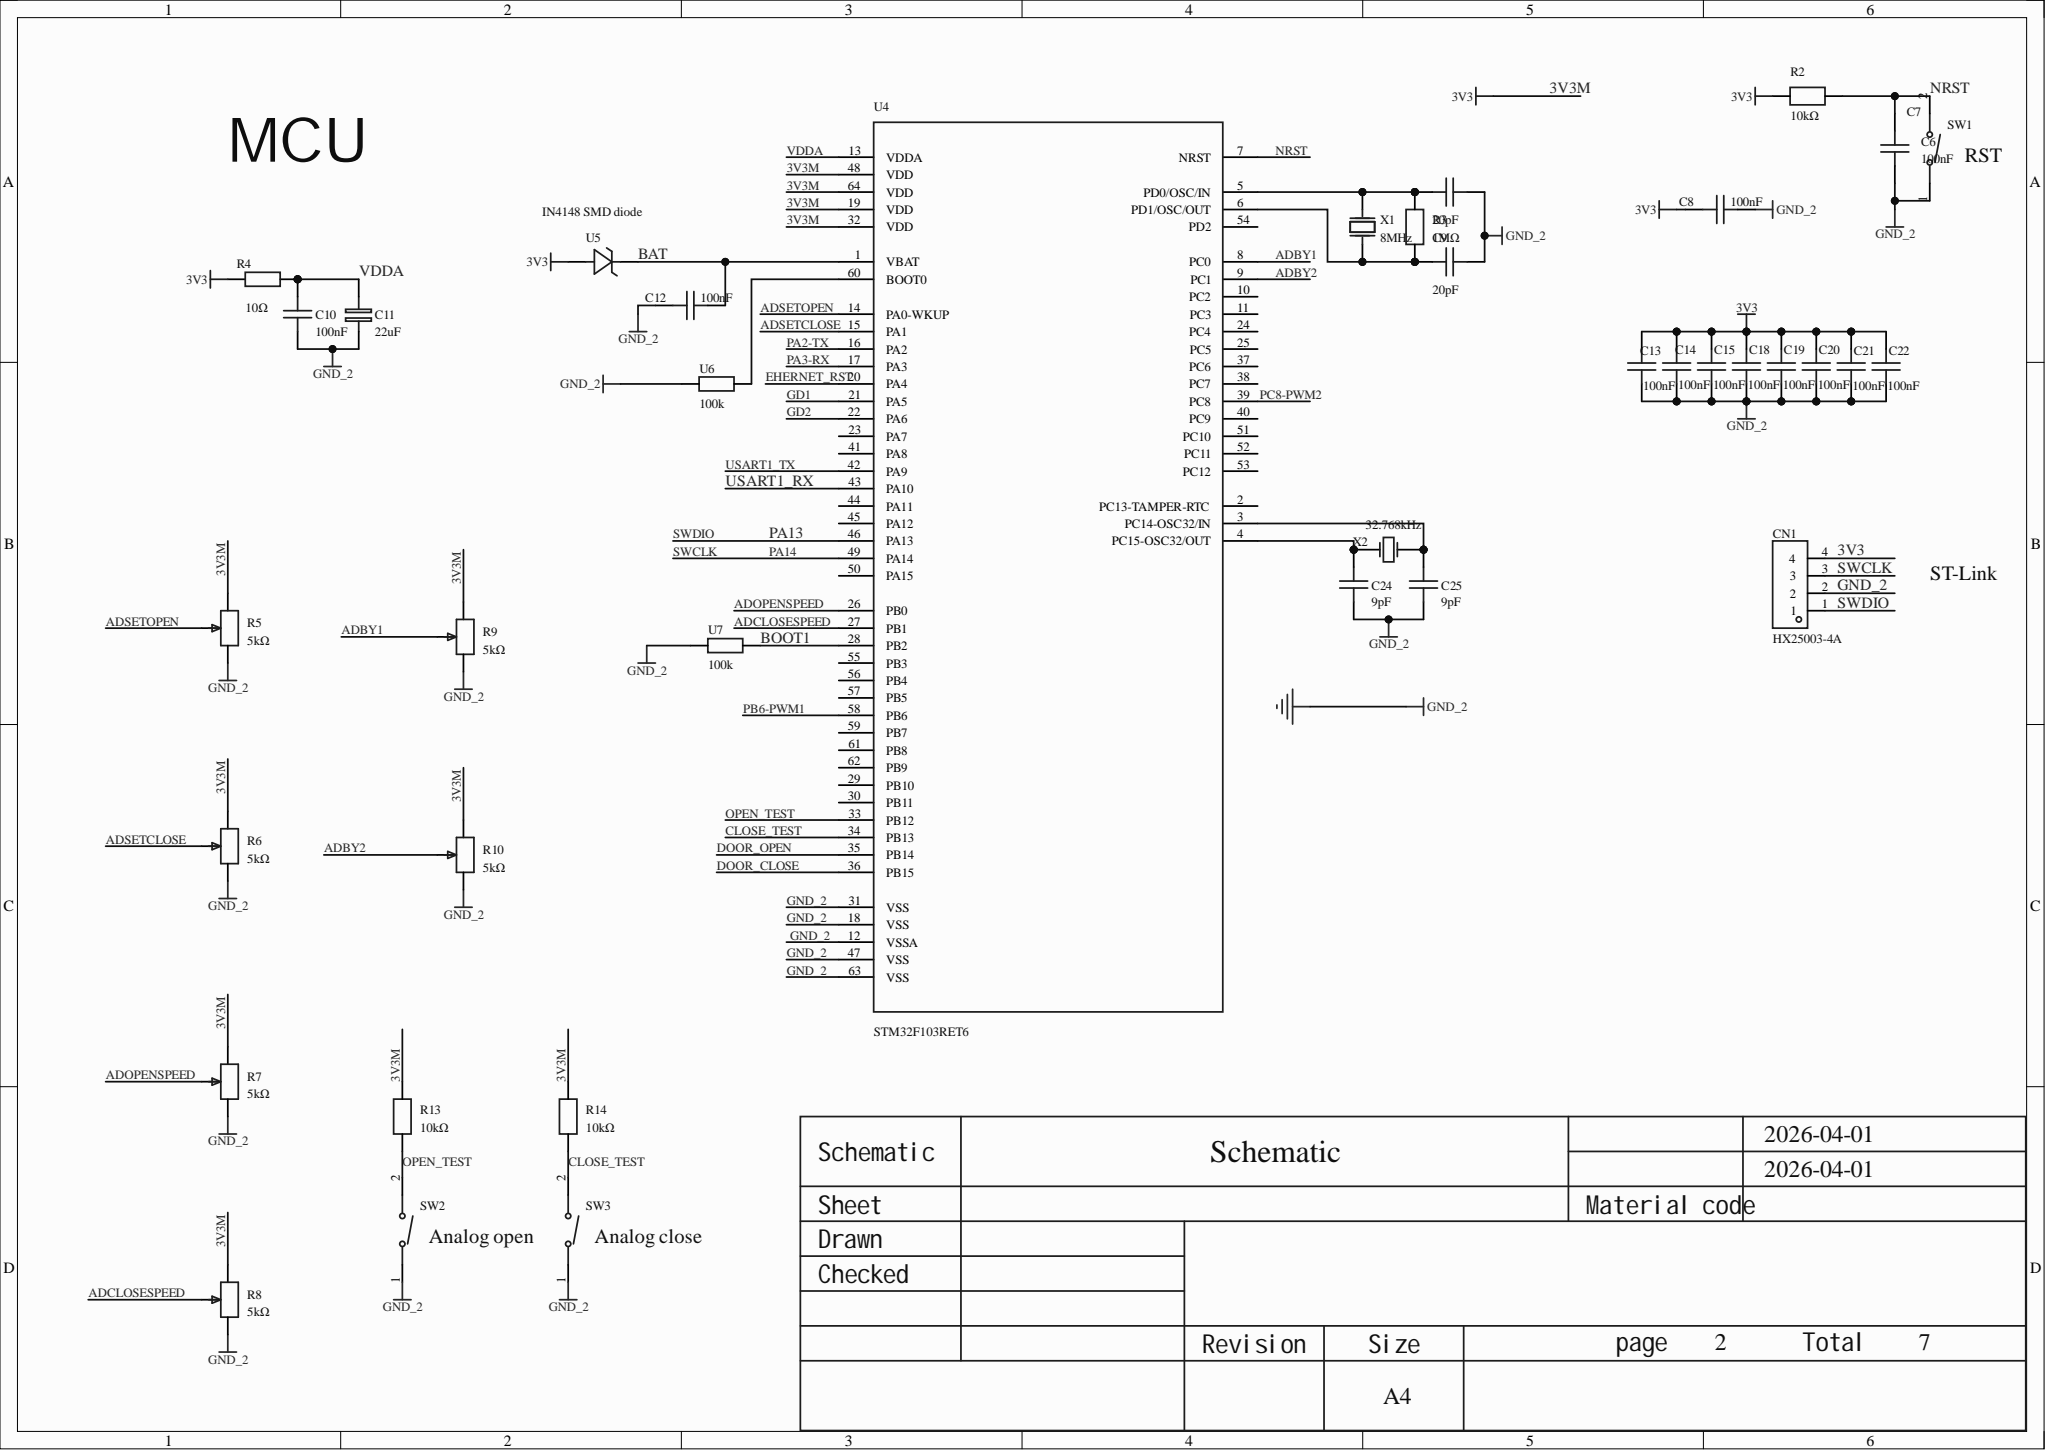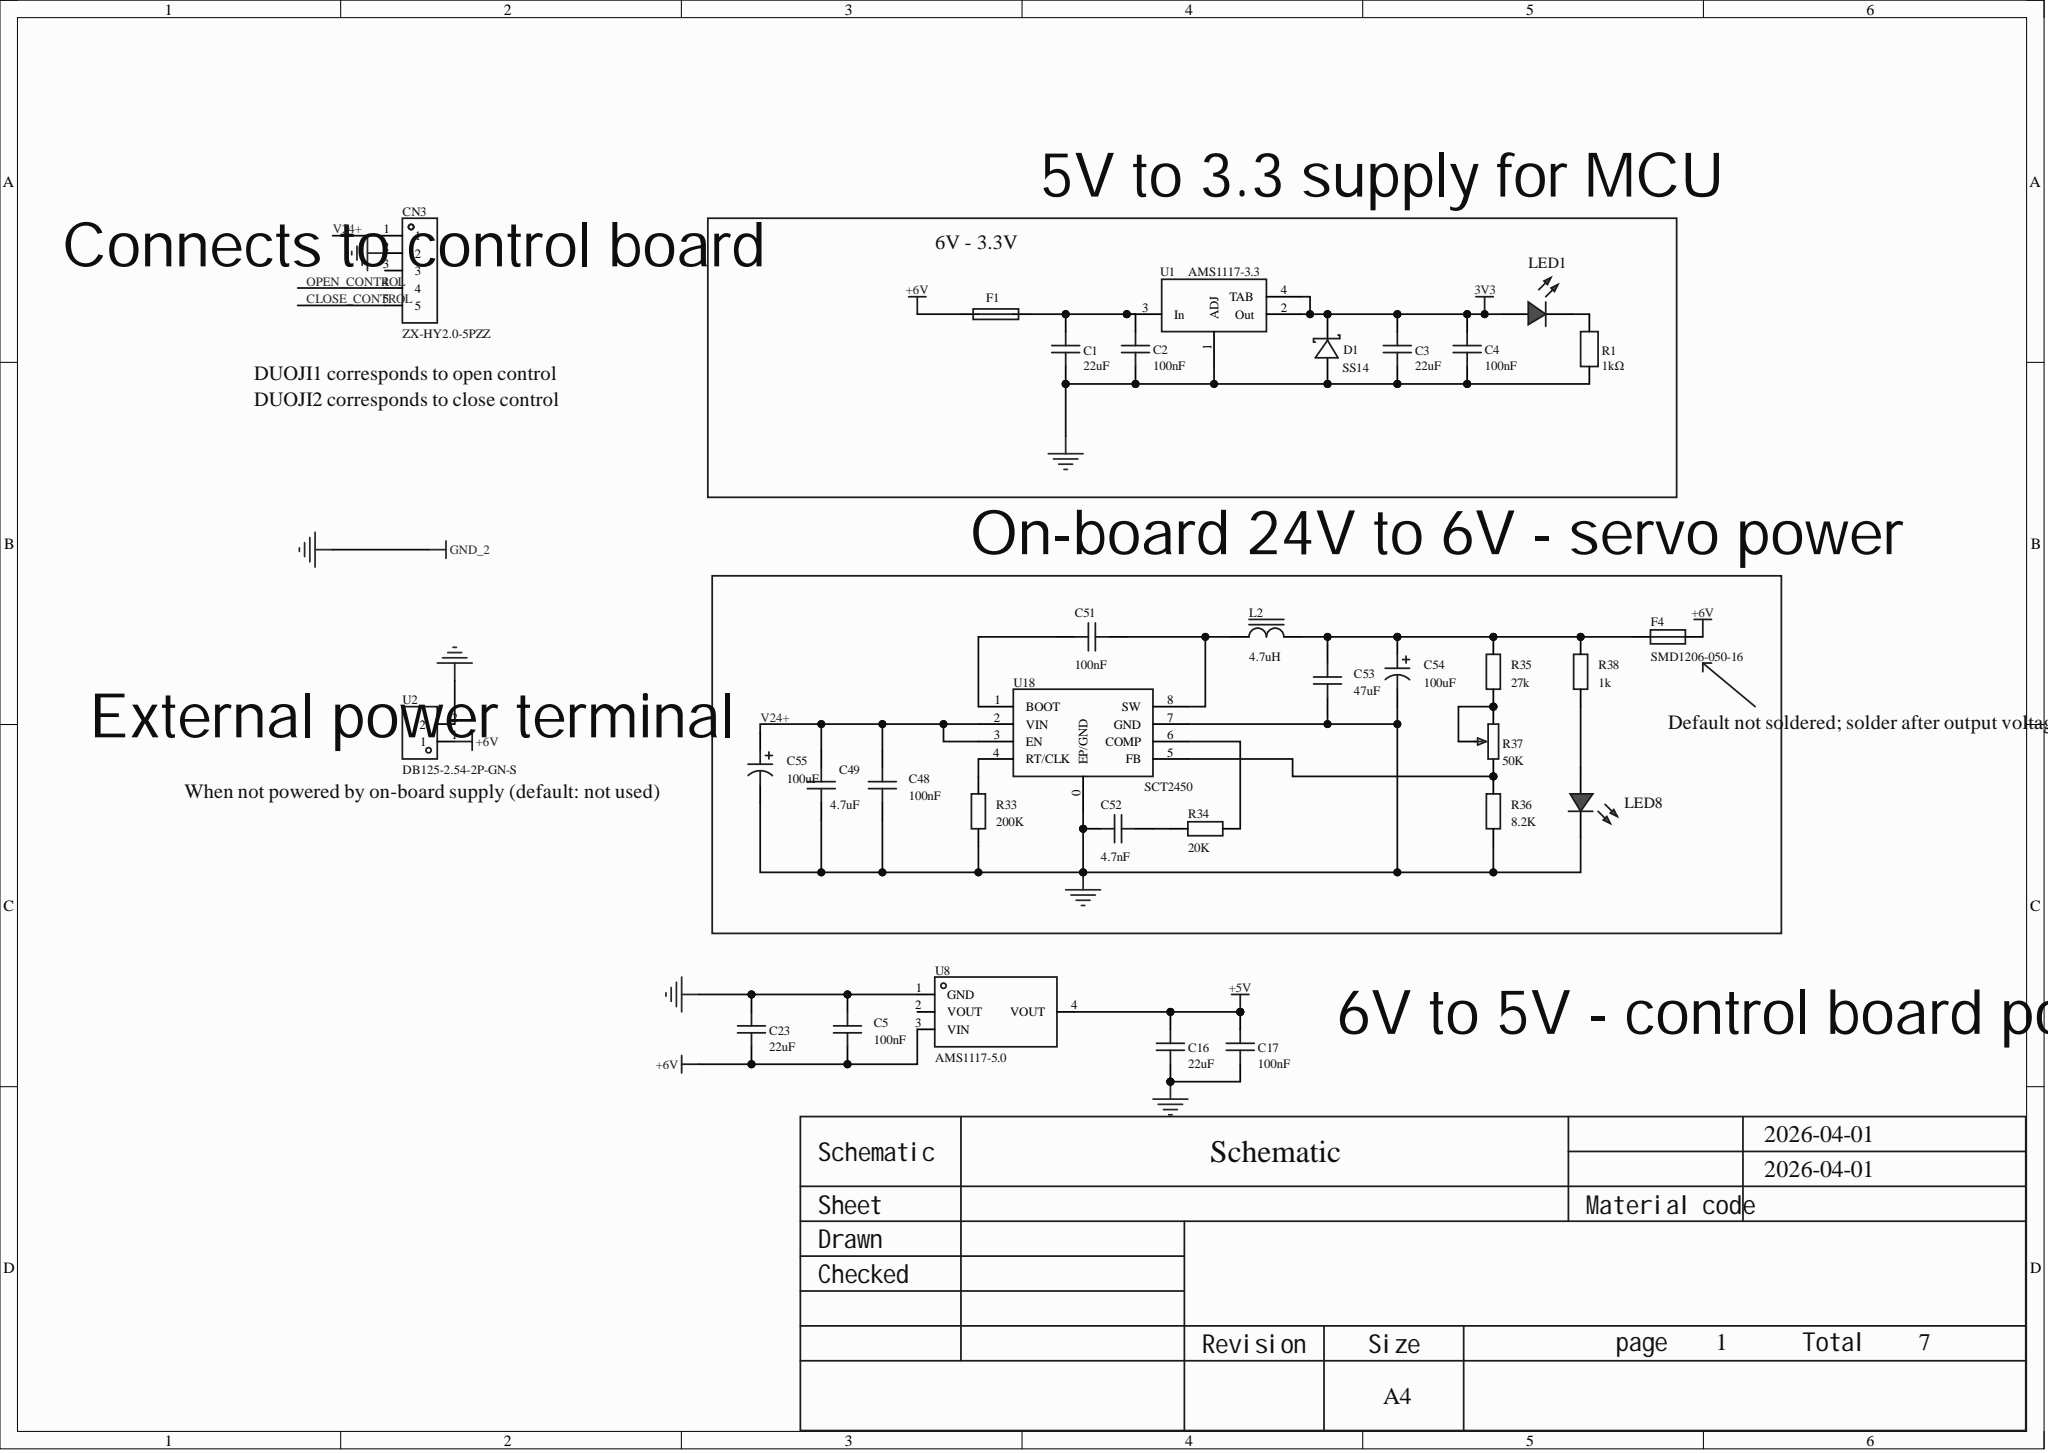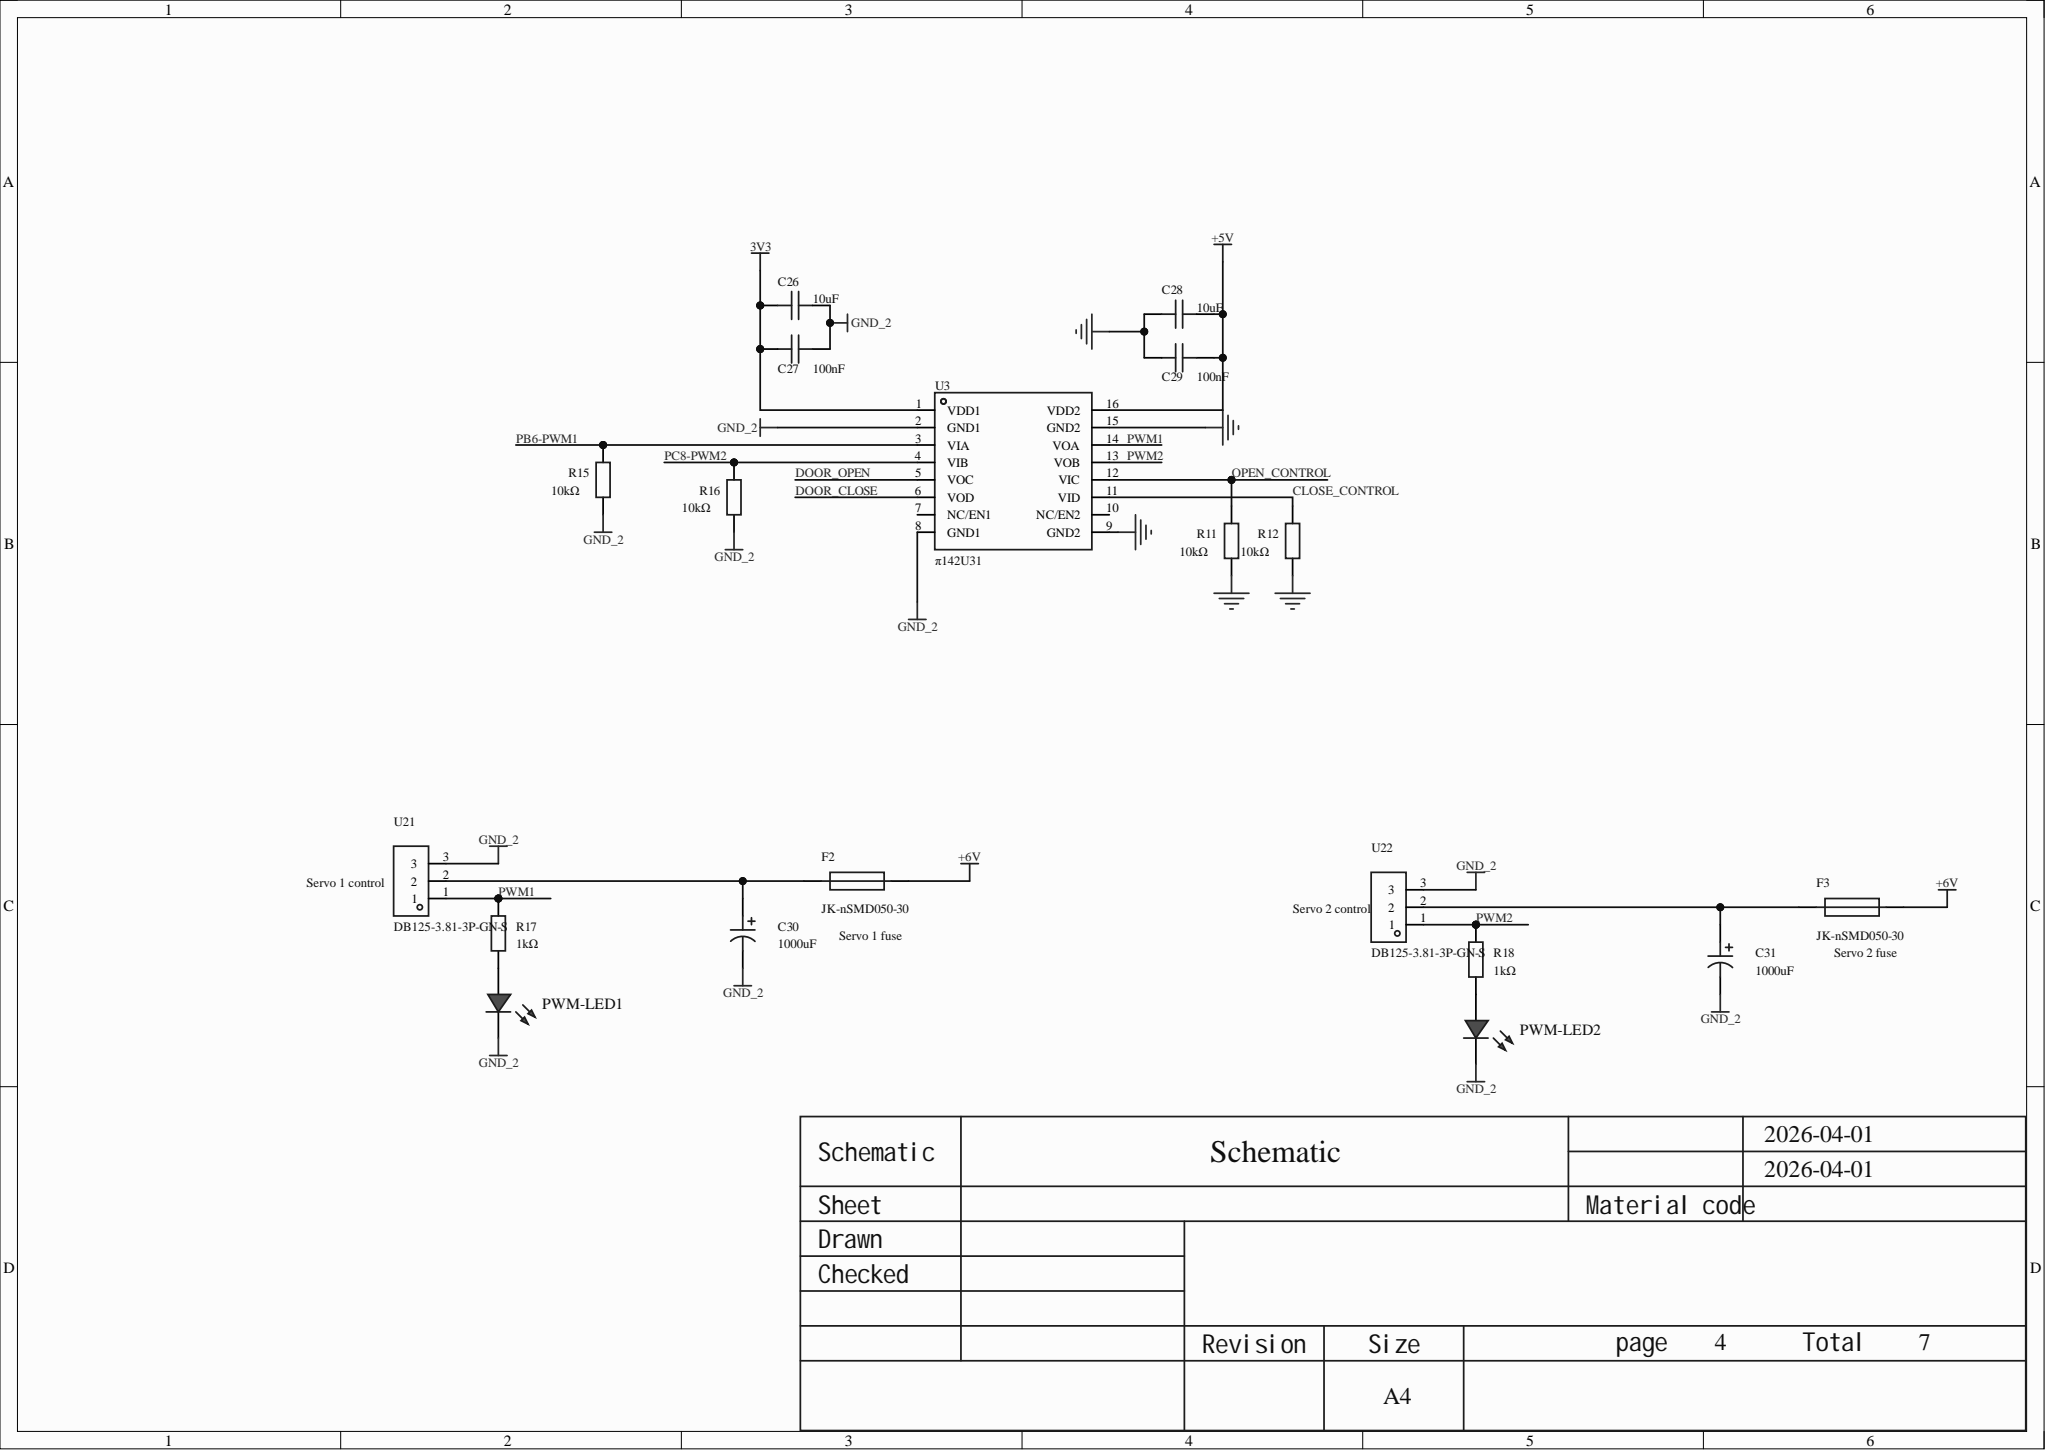Circuit board | Altium Designer | 90 parts | 47 nets
Bill of materials:
Comment,Description,Designator,Footprint,LibRef,Quantity
"22uF","Capacitance: 22uF; tolerance: ±20%; rated voltage: 6.3V; dielectric (temp. coefficient): X5R;","C1, C3, C11, C16, C23","C0603","CL10A226MQ8NRNC","5"
"100nF","Capacitance: 100nF; tolerance: ±10%; rated voltage: 50V; dielectric (temp. coefficient): X7R;, [NoValue]","C2, C4, C5, C6, C8, C10, C12, C13, C14, C15, C17, C18, C19, C20, C21, C22, C27, C29, C48, C51","C0603","CC0603KRX7R9BB104, CAP_0603","20"
"20pF","Capacitance: 20pF; tolerance: ±5%; rated voltage: 50V; dielectric (temp. coefficient): NP0;","C7, C9","C0603","CC0603JRNPO9BN200","2"
"9pF","Capacitance: 9pF; rated voltage: 50V; dielectric (temp. coefficient): C0G;","C24, C25","C0402","0402CG9R0C500NT","2"
"10uF","Capacitance: 10uF; tolerance: ±10%; rated voltage: 50V; dielectric (temp. coefficient): X5R;","C26, C28","C0805","GRM21BR61H106KE43L","2"
"1000uF","Capacitance: 1000uF; tolerance: ±20%; rated voltage: 6.3V;","C30, C31","CAP-TH_BD6.3-P2.50-D0.5-FD","SPZ0JM102E10C35RAXXX","2"
"4.7uF","","C49","C0603","CAP_0603","1"
"4.7nF","","C52","C0603","CAP_0603","1"
"47uF","","C53","C0603","CAP_0603","1"
"100uF","Capacitance: 100uF; rated voltage: 16V;","C54, C55","CAP-TH_BD5.0-P2.00-D0.5-FD","1010160507R00","2"
"HX25003-4A","Pin structure: 1x4P; pitch: 2.5mm; gender: male; mounting: through-hole; row spacing: -; rows: 1; pins per row: 4; reference series: XH; rated current: -; operating temperature range: -;","CN1","CONN-TH_4P-P2.50_HX25003-4A","HX25003-4A","1"
"ZX-HY2.0-5PZZ","插针结构:1x5P;间距:2mm;安装方式:直插;参考系列:HY;总PIN数:5P;排数:1;每排PIN数:5;行距:-;额定电流:2A;触头材质:黄铜;触头镀层:锡;工作温度范围:-25℃~+85℃;","CN3","CONN-TH_5P-P2.00_ZX-HY2.0-5PZZ","ZX-HY2.0-5PZZ","1"
"SS14","Diode configuration: single; forward voltage (Vf): 550mV@1A; DC reverse voltage (Vr): 40V; average rectified current (Io): 1A;","D1","SMA_L4.2-W2.6-LS5.3-RD","SS14_C2480","1"
"PICOSMDC050S-2","Max voltage: 6V; max current: 100A; hold current: 500mA; trip current: 1A;","F1","F0805","PICOSMDC050S-2","1"
"JK-nSMD050-30","Max voltage: 30V; max current: 100A; hold current: 500mA; trip current: 1A;","F2, F3","F1206","JK-nSMD050-30","2"
"SMD1206-050-16","Withstand voltage (Vmax): 16V; max current (Imax): 40A; hold current (Ihold): 500mA; trip current (Itrip): 1A;","F4","F1206","SMD1206-050-16","1"
"4.7uH","","L2","0630 TPC 7*7*3","Ind-Power","1"
"","","LED1, LED8, PWM-LED1, PWM-LED2","LED_0603","LED_0603-R","4"
"1kΩ","Resistance: 1kΩ; tolerance: ±1%; power: 100mW; temp. coefficient: ±100ppm/?; resistor type: thick film resistor;","R1, R17, R18","R0603","0603WAF1001T5E","3"
"10kΩ","Resistance: 10kΩ; tolerance: ±1%; power: 100mW; temp. coefficient: ±100ppm/?; resistor type: thick film resistor;, Resistor type: thick film resistor; resistance: 3.3kΩ; tolerance: ±1%; power: 100mW; max working voltage: 75V; temp. coefficient: ±100ppm/?;","R2, R11, R12, R13, R14, R15, R16","R0603","0603WAF1002T5E, 0603WAF3301T5E","7"
"1MΩ","Resistance: 1MΩ; tolerance: ±1%; power: 100mW; temp. coefficient: ±100ppm/?; resistor type: thick film resistor;","R3","R0603","0603WAF1004T5E","1"
"10Ω","Resistance: 10Ω; tolerance: ±1%; power: 100mW; temp. coefficient: ±400ppm/?; resistor type: thick film resistor;","R4","R0603","0603WAF100JT5E","1"
"5kΩ","Resistance: 5kΩ; tolerance: ±10%; power: 500mW; temp. coefficient: ±250ppm/?;","R5, R6, R7, R8, R9, R10","RES-ADJ-TH_3296W-1-203","3296W-1-502_C48997929","6"
"200K","","R33","R0603","Res_0603","1"
"20K","","R34","R0603","Res_0603","1"
"27k","","R35","R0603","Res_0603","1"
"8.2K","","R36","R0603","Res_0603","1"
"50K","","R37","RESPOT3296","Res-Adj-3p","1"
"1k","","R38","R0603","Res_0603","1"
"TS-1101-C-W","电路结构:单刀单掷;带支架:否;触点电流:50mA;额定电压(AC):-;额定电压(DC):12V;额定功率:-;安装方式:立贴;绝缘电阻:-;带灯:无;作用力:260gf;机械寿命:5万次;","SW1, SW2, SW3","SW-SMD_L6.0-W3.3-LS8.0","TS-1101-C-W","3"
"AMS1117-3.3","Output type: fixed; max input voltage: -; output voltage: 3.3V; output current: 1A; PSRR: 72dB@(120Hz); output polarity: positive;","U1","SOT-223-3_L6.5-W3.4-P2.30-LS7.0-BR","AMS1117-3.3_C6186","1"
"DB125-2.54-2P-GN-S","结构:1x2P;间距:2.54mm;颜色:绿色;安装方式:直插;排数:1;每排PIN数:2;额定电流:7A;额定电压:150V;线规 - AWG:18~26;线规 - 平方毫米:1;工作温度:-40℃~+105℃;","U2","CONN-TH_DB125-2.54-2P-GN","DB125-2.54-2P-GN-S","1"
"p142U31","通过使用成熟的标准半导体CMOS技术和iDivider技术，这些隔离组件提供了出色的性能特性和可靠性，优于光耦设备和其他集成隔离器等替代产品。智能分压器技术（iDivider技术）是一种新一代数字隔离器技术，它利用电容分压器原理直接跨隔离器电容传输电压信号，无需信号调制和解调。隔离器数据通道独立，有多种配置可供选择，耐压额定值为1.5kV rms至6.0kV rms，数据速率从直流到600Mbps。设备两侧的电源电压范围为3.0V至5.5V，可与低电压系统兼容，并能在隔离屏障上实现电压转换功能。当未施加输","U3","SOIC-16_L9.9-W3.9-P1.27-LS6.0-BL","p142U31","1"
"STM32F103RET6","CPU core: CM3; program memory: 512KB; total RAM: 64KB; GPIO ports: 51; operating voltage: 2V~3.6V; max CPU frequency: 72MHz; program memory type: FLASH;","U4","LQFP-64_L10.0-W10.0-P0.50-LS12.0-BL","STM32F103RET6","1"
"IN4148 SMD diode","","U5","SOD-123_L2.7-W1.7-LS3.8-RD","IN4148贴片二极管","1"
"100k","","U6, U7","R0603","100k","2"
"AMS1117-5.0","Output type: fixed; operating voltage: 15V; output voltage: 5V; output current: 1A; PSRR: 60dB; output polarity: positive;","U8","SOT-223_L6.5-W3.5-P2.30-LS7.0-BR","AMS1117-5.0_C6187","1"
"SCT2450","","U18","SOP-8E","SCT2450","1"
"DB125-3.81-3P-GN-S","结构:1x3P;间距:3.81mm;颜色:绿色;安装方式:直插;额定电流:10A;额定电压:300V;排数:1;线规 - AWG:16~26;线规 - 平方毫米:0.5~1;每排PIN数:3;工作温度范围:-40℃~+105℃;","U21, U22","CONN-TH_3P-P3.81_L7.4-W11.4","DB125-3.81-3P-GN-S","2"
"8MHz","Frequency: 8MHz; load capacitance: 20pF; frequency tolerance: ±20ppm;","X1","CRYSTAL-SMD_L11.5-W4.8-LS12.7","X49SM8MSD2SC","1"
"32.768kHz","Frequency: 32.768kHz; load capacitance: 12.5pF; frequency tolerance: ±20ppm;","X2","OSC-SMD_L3.2-W1.5","SC-32S32.768kHz20PPM12.5pF","1"
Netlist (Protel format):
[
C1
C0603
22uF



]
[
C2
C0603
100nF



]
[
C3
C0603
22uF



]
[
C4
C0603
100nF



]
[
C5
C0603
100nF



]
[
C6
C0603
100nF



]
[
C7
C0603
20pF



]
[
C8
C0603
100nF



]
[
C9
C0603
20pF



]
[
C10
C0603
100nF



]
[
C11
C0603
22uF



]
[
C12
C0603
100nF



]
[
C13
C0603
100nF



]
[
C14
C0603
100nF



]
[
C15
C0603
100nF



]
[
C16
C0603
22uF



]
[
C17
C0603
100nF



]
[
C18
C0603
100nF



]
[
C19
C0603
100nF



]
[
C20
C0603
100nF



]
[
C21
C0603
100nF



]
[
C22
C0603
100nF



]
[
C23
C0603
22uF



]
[
C24
C0402
9pF



]
[
C25
C0402
9pF



]
[
C26
C0805
10uF



]
[
C27
C0603
100nF



]
[
C28
C0805
10uF



]
[
C29
C0603
100nF



]
[
C30
CAP-TH_BD6.3-P2.50-D0.5-FD
1000uF



]
[
C31
CAP-TH_BD6.3-P2.50-D0.5-FD
1000uF



]
[
C48
C0603
100nF



]
[
C49
C0603
4.7uF



]
[
C51
C0603
100nF



]
[
C52
C0603
4.7nF



]
[
C53
C0603
47uF



]
[
C54
CAP-TH_BD5.0-P2.00-D0.5-FD
100uF



]
[
C55
CAP-TH_BD5.0-P2.00-D0.5-FD
100uF



]
[
CN1
CONN-TH_4P-P2.50_HX25003-4A
HX25003-4A



]
[
CN3
CONN-TH_5P-P2.00_ZX-HY2.0-5PZZ
ZX-HY2.0-5PZZ



]
[
D1
SMA_L4.2-W2.6-LS5.3-RD
SS14



]
[
F1
F0805
PICOSMDC050S-2



]
[
F2
F1206
JK-nSMD050-30



]
[
F3
F1206
JK-nSMD050-30



]
[
F4
F1206
SMD1206-050-16



]
[
L2
0630 TPC 7*7*3
4.7uH



]
[
LED1
LED_0603




]
[
LED8
LED_0603




]
[
PWM-LED1
LED_0603




]
[
PWM-LED2
LED_0603




]
[
R1
R0603
1kΩ



]
[
R2
R0603
10kΩ



]
[
R3
R0603
1MΩ



]
[
R4
R0603
10Ω



]
[
R5
RES-ADJ-TH_3296W-1-203
5kΩ



]
[
R6
RES-ADJ-TH_3296W-1-203
5kΩ



]
[
R7
RES-ADJ-TH_3296W-1-203
5kΩ



]
[
R8
RES-ADJ-TH_3296W-1-203
5kΩ



]
[
R9
RES-ADJ-TH_3296W-1-203
5kΩ



]
[
R10
RES-ADJ-TH_3296W-1-203
5kΩ



]
[
R11
R0603
10kΩ



]
[
R12
R0603
10kΩ



]
[
R13
R0603
10kΩ



]
[
R14
R0603
10kΩ



]
[
R15
R0603
10kΩ



]
[
R16
R0603
10kΩ



]
[
R17
R0603
1kΩ



]
[
R18
R0603
1kΩ



]
[
R33
R0603
200K



]
[
R34
R0603
20K



]
[
R35
R0603
27k



]
[
R36
R0603
8.2K



]
[
R37
RESPOT3296
50K



]
[
R38
R0603
1k



]
[
SW1
SW-SMD_L6.0-W3.3-LS8.0
TS-1101-C-W



]
[
SW2
SW-SMD_L6.0-W3.3-LS8.0
TS-1101-C-W



]
[
SW3
SW-SMD_L6.0-W3.3-LS8.0
TS-1101-C-W



]
[
U1
SOT-223-3_L6.5-W3.4-P2.30-LS7.0-BR
AMS1117-3.3



]
[
U2
CONN-TH_DB125-2.54-2P-GN
DB125-2.54-2P-GN-S



]
[
U3
SOIC-16_L9.9-W3.9-P1.27-LS6.0-BL
p142U31



]
[
U4
LQFP-64_L10.0-W10.0-P0.50-LS12.0-BL
STM32F103RET6



]
[
U5
SOD-123_L2.7-W1.7-LS3.8-RD
IN4148 SMD diode



]
[
U6
R0603
100k



]
[
U7
R0603
100k



]
[
U8
SOT-223_L6.5-W3.5-P2.30-LS7.0-BR
AMS1117-5.0



]
[
U18
SOP-8E
SCT2450



]
[
U21
CONN-TH_3P-P3.81_L7.4-W11.4
DB125-3.81-3P-GN-S



]
[
U22
CONN-TH_3P-P3.81_L7.4-W11.4
DB125-3.81-3P-GN-S



]
[
X1
CRYSTAL-SMD_L11.5-W4.8-LS12.7
8MHz



]
[
X2
OSC-SMD_L3.2-W1.5
32.768kHz



]
(
VDDA
C10-2
C11-2
R4-2
U4-13
)
(
V24+
C48-2
C49-2
C55-1
CN3-1
U18-2
U18-3
)
(
PWM2
R18-2
U3-13
U22-1
)
(
PWM1
R17-2
U3-14
U21-1
)
(
PC8-PWM2
R16-2
U3-4
U4-39
)
(
PB6-PWM1
R15-2
U3-3
U4-58
)
(
PA14
CN1-3
U4-49
)
(
PA13
CN1-1
U4-46
)
(
OPEN_TEST
R13-2
SW2-2
U4-33
)
(
OPEN_CONTROL
CN3-4
R11-2
U3-12
)
(
NRST
C6-1
R2-2
SW1-2
U4-7
)
(
NetU4_60
U4-60
U6-1
)
(
NetR36_2
R36-2
R37-2
U18-5
)
(
NetR35_1
R35-1
R37-1
R37-ADJ
)
(
NetR34_1
R34-1
U18-6
)
(
NetR33_2
R33-2
U18-4
)
(
NetPWM-LED2_2
PWM-LED2-2
R18-1
)
(
NetPWM-LED1_2
PWM-LED1-2
R17-1
)
(
NetLED8_2
LED8-2
R38-1
)
(
NetLED1_1
LED1-1
R1-2
)
(
NetC53_1
C53-1
C54-1
F4-1
L2-2
R35-2
R38-2
)
(
NetC52_1
C52-1
R34-2
)
(
NetC51_2
C51-2
U18-1
)
(
NetC51_1
C51-1
L2-1
U18-8
)
(
NetC31_1
C31-1
F3-1
U22-2
)
(
NetC30_1
C30-1
F2-1
U21-2
)
(
NetC25_2
C25-2
U4-3
X2-1
)
(
NetC24_2
C24-2
U4-4
X2-2
)
(
NetC9_2
C9-2
R3-2
U4-6
X1-2
)
(
NetC7_2
C7-2
R3-1
U4-5
X1-1
)
(
NetC1_2
C1-2
C2-2
F1-2
U1-3
)
(
GND_2
C1-1
C2-1
C3-1
C4-1
C5-2
C6-2
C7-1
C8-2
C9-1
C10-1
C11-1
C12-1
C13-1
C14-1
C15-1
C16-1
C17-1
C18-1
C19-1
C20-1
C21-1
C22-1
C23-2
C24-1
C25-1
C26-2
C27-1
C28-1
C29-2
C30-2
C31-2
C48-1
C49-1
C52-2
C53-2
C54-2
C55-2
CN1-2
CN3-2
D1-2
LED8-1
PWM-LED1-1
PWM-LED2-1
R1-1
R5-1
R6-1
R7-1
R8-1
R9-1
R10-1
R11-1
R12-1
R15-1
R16-1
R33-1
R36-1
SW1-1
SW2-1
SW3-1
U1-1
U2-2
U3-2
U3-8
U3-9
U3-15
U4-12
U4-18
U4-31
U4-47
U4-63
U6-2
U7-1
U8-1
U18-0
U18-7
U21-3
U22-3
)
(
DOOR_OPEN
U3-5
U4-35
)
(
DOOR_CLOSE
U3-6
U4-36
)
(
CLOSE_TEST
R14-2
SW3-2
U4-34
)
(
CLOSE_CONTROL
CN3-5
R12-2
U3-11
)
(
BOOT1
U4-28
U7-2
)
(
BAT
C12-2
U4-1
U5-1
)
(
ADSETOPEN
R5-2
U4-14
)
(
ADSETCLOSE
R6-2
U4-15
)
(
ADOPENSPEED
R7-2
U4-26
)
(
ADCLOSESPEED
R8-2
U4-27
)
(
ADBY2
R10-2
U4-9
)
(
ADBY1
R9-2
U4-8
)
(
+6V
C5-1
C23-1
F1-1
F2-2
F3-2
F4-2
U2-1
U8-3
)
(
+5V
C16-2
C17-2
C28-2
C29-1
U3-16
U8-4
)
(
3V3
C3-2
C4-2
C8-1
C13-2
C14-2
C15-2
C18-2
C19-2
C20-2
C21-2
C22-2
C26-1
C27-2
CN1-4
D1-1
LED1-2
R2-1
R4-1
R5-3
R6-3
R7-3
R8-3
R9-3
R10-3
R13-1
R14-1
U1-2
U1-4
U3-1
U4-19
U4-32
U4-48
U4-64
U5-2
)